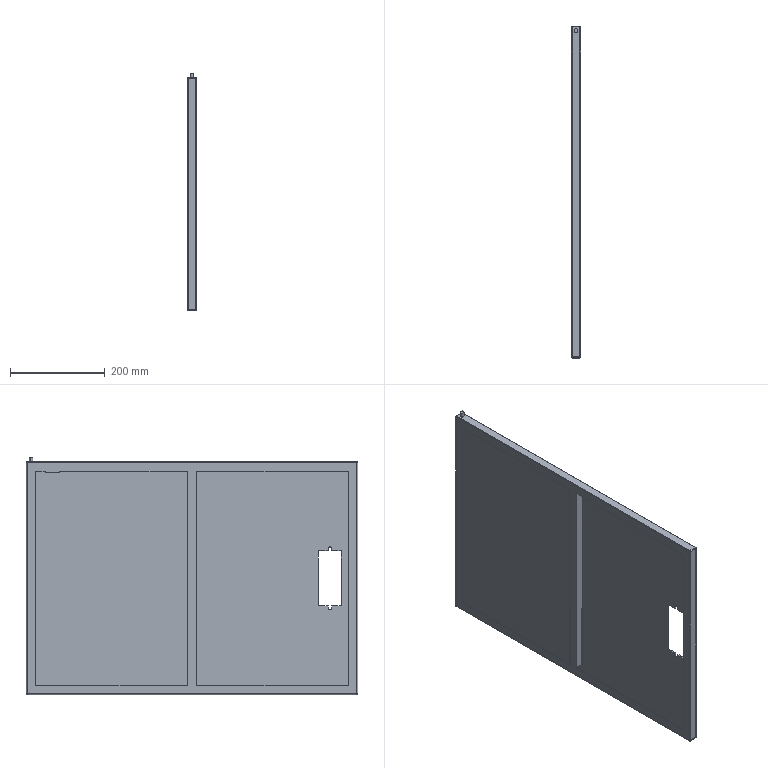Part | STEP file | Lower frame door panel | 1 solid | 69 faces | box 20 x 700 x 502 mm | volume 890062 mm3 | plane 42 | cylinder 19 | sphere 8 | commonest cylinder face diameters 4 x12 7 x3 3.3 x2 8 x2